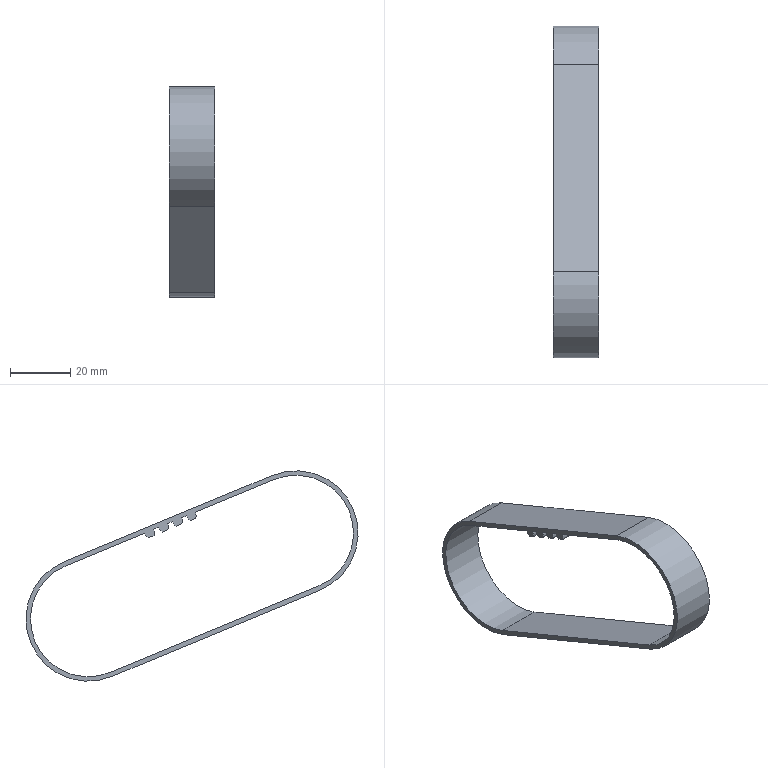Part | NX | features 5003_013_C-HTBN270S5M-150(Default) 2 | 1 solid | 26 faces | box 15 x 109.992 x 69.695 mm | volume 6484 mm3 | plane 14 | cylinder 12 | commonest cylinder face diameters 6.5 x8 38.2 x2 41.2 x2
STEP:
#1=CARTESIAN_POINT('',(-7.975,102.341,-117.355));
#2=VERTEX_POINT('',#1);
#3=CARTESIAN_POINT('',(7.025,102.341,-117.355));
#4=VERTEX_POINT('',#3);
#5=CARTESIAN_POINT('',(-7.975,102.341,-117.355));
#6=DIRECTION('',(1.,0.,0.));
#7=VECTOR('',#6,1000.);
#8=LINE('',#5,#7);
#9=EDGE_CURVE('',#2,#4,#8,.T.);
#10=ORIENTED_EDGE('',*,*,#9,.T.);
#11=CARTESIAN_POINT('',(7.025,100.724,-116.685));
#12=VERTEX_POINT('',#11);
#13=CARTESIAN_POINT('',(7.025,62.517,-100.859));
#14=DIRECTION('',(0.,-0.9239,0.3827));
#15=VECTOR('',#14,1000.);
#16=LINE('',#13,#15);
#17=EDGE_CURVE('',#4,#12,#16,.T.);
#18=ORIENTED_EDGE('',*,*,#17,.T.);
#19=CARTESIAN_POINT('',(-7.975,100.724,-116.685));
#20=VERTEX_POINT('',#19);
#21=CARTESIAN_POINT('',(-7.975,100.724,-116.685));
#22=DIRECTION('',(1.,0.,0.));
#23=VECTOR('',#22,1000.);
#24=LINE('',#21,#23);
#25=EDGE_CURVE('',#20,#12,#24,.T.);
#26=ORIENTED_EDGE('',*,*,#25,.F.);
#27=CARTESIAN_POINT('',(-7.975,62.517,-100.859));
#28=DIRECTION('',(0.,-0.9239,0.3827));
#29=VECTOR('',#28,1000.);
#30=LINE('',#27,#29);
#31=EDGE_CURVE('',#2,#20,#30,.T.);
#32=ORIENTED_EDGE('',*,*,#31,.F.);
#33=EDGE_LOOP('',(#10,#18,#26,#32));
#34=FACE_BOUND('',#33,.T.);
#35=CARTESIAN_POINT('',(7.025,62.517,-100.859));
#36=DIRECTION('',(0.,-0.3827,-0.9239));
#37=DIRECTION('',(-1.,0.,0.));
#38=AXIS2_PLACEMENT_3D('',#35,#36,#37);
#39=PLANE('',#38);
#40=ADVANCED_FACE('',(#34),#39,.T.);
#41=CARTESIAN_POINT('',(-7.975,97.722,-115.441));
#42=VERTEX_POINT('',#41);
#43=CARTESIAN_POINT('',(7.025,97.722,-115.441));
#44=VERTEX_POINT('',#43);
#45=CARTESIAN_POINT('',(-7.975,97.722,-115.441));
#46=DIRECTION('',(1.,0.,0.));
#47=VECTOR('',#46,1000.);
#48=LINE('',#45,#47);
#49=EDGE_CURVE('',#42,#44,#48,.T.);
#50=ORIENTED_EDGE('',*,*,#49,.T.);
#51=CARTESIAN_POINT('',(7.025,96.105,-114.772));
#52=VERTEX_POINT('',#51);
#53=CARTESIAN_POINT('',(7.025,62.517,-100.859));
#54=DIRECTION('',(0.,-0.9239,0.3827));
#55=VECTOR('',#54,1000.);
#56=LINE('',#53,#55);
#57=EDGE_CURVE('',#44,#52,#56,.T.);
#58=ORIENTED_EDGE('',*,*,#57,.T.);
#59=CARTESIAN_POINT('',(-7.975,96.105,-114.772));
#60=VERTEX_POINT('',#59);
#61=CARTESIAN_POINT('',(-7.975,96.105,-114.772));
#62=DIRECTION('',(1.,0.,0.));
#63=VECTOR('',#62,1000.);
#64=LINE('',#61,#63);
#65=EDGE_CURVE('',#60,#52,#64,.T.);
#66=ORIENTED_EDGE('',*,*,#65,.F.);
#67=CARTESIAN_POINT('',(-7.975,62.517,-100.859));
#68=DIRECTION('',(0.,-0.9239,0.3827));
#69=VECTOR('',#68,1000.);
#70=LINE('',#67,#69);
#71=EDGE_CURVE('',#42,#60,#70,.T.);
#72=ORIENTED_EDGE('',*,*,#71,.F.);
#73=EDGE_LOOP('',(#50,#58,#66,#72));
#74=FACE_BOUND('',#73,.T.);
#75=CARTESIAN_POINT('',(7.025,62.517,-100.859));
#76=DIRECTION('',(0.,-0.3827,-0.9239));
#77=DIRECTION('',(-1.,0.,0.));
#78=AXIS2_PLACEMENT_3D('',#75,#76,#77);
#79=PLANE('',#78);
#80=ADVANCED_FACE('',(#74),#79,.T.);
#81=CARTESIAN_POINT('',(-7.975,93.102,-113.528));
#82=VERTEX_POINT('',#81);
#83=CARTESIAN_POINT('',(7.025,93.102,-113.528));
#84=VERTEX_POINT('',#83);
#85=CARTESIAN_POINT('',(-7.975,93.102,-113.528));
#86=DIRECTION('',(1.,0.,0.));
#87=VECTOR('',#86,1000.);
#88=LINE('',#85,#87);
#89=EDGE_CURVE('',#82,#84,#88,.T.);
#90=ORIENTED_EDGE('',*,*,#89,.T.);
#91=CARTESIAN_POINT('',(7.025,91.485,-112.858));
#92=VERTEX_POINT('',#91);
#93=CARTESIAN_POINT('',(7.025,62.517,-100.859));
#94=DIRECTION('',(0.,-0.9239,0.3827));
#95=VECTOR('',#94,1000.);
#96=LINE('',#93,#95);
#97=EDGE_CURVE('',#84,#92,#96,.T.);
#98=ORIENTED_EDGE('',*,*,#97,.T.);
#99=CARTESIAN_POINT('',(-7.975,91.485,-112.858));
#100=VERTEX_POINT('',#99);
#101=CARTESIAN_POINT('',(-7.975,91.485,-112.858));
#102=DIRECTION('',(1.,0.,0.));
#103=VECTOR('',#102,1000.);
#104=LINE('',#101,#103);
#105=EDGE_CURVE('',#100,#92,#104,.T.);
#106=ORIENTED_EDGE('',*,*,#105,.F.);
#107=CARTESIAN_POINT('',(-7.975,62.517,-100.859));
#108=DIRECTION('',(0.,-0.9239,0.3827));
#109=VECTOR('',#108,1000.);
#110=LINE('',#107,#109);
#111=EDGE_CURVE('',#82,#100,#110,.T.);
#112=ORIENTED_EDGE('',*,*,#111,.F.);
#113=EDGE_LOOP('',(#90,#98,#106,#112));
#114=FACE_BOUND('',#113,.T.);
#115=CARTESIAN_POINT('',(7.025,62.517,-100.859));
#116=DIRECTION('',(0.,-0.3827,-0.9239));
#117=DIRECTION('',(-1.,0.,0.));
#118=AXIS2_PLACEMENT_3D('',#115,#116,#117);
#119=PLANE('',#118);
#120=ADVANCED_FACE('',(#114),#119,.T.);
#121=CARTESIAN_POINT('',(-7.975,88.483,-111.615));
#122=VERTEX_POINT('',#121);
#123=CARTESIAN_POINT('',(7.025,88.483,-111.615));
#124=VERTEX_POINT('',#123);
#125=CARTESIAN_POINT('',(-7.975,88.483,-111.615));
#126=DIRECTION('',(1.,0.,0.));
#127=VECTOR('',#126,1000.);
#128=LINE('',#125,#127);
#129=EDGE_CURVE('',#122,#124,#128,.T.);
#130=ORIENTED_EDGE('',*,*,#129,.T.);
#131=CARTESIAN_POINT('',(7.025,62.517,-100.859));
#132=VERTEX_POINT('',#131);
#133=CARTESIAN_POINT('',(7.025,62.517,-100.859));
#134=DIRECTION('',(0.,-0.9239,0.3827));
#135=VECTOR('',#134,1000.);
#136=LINE('',#133,#135);
#137=EDGE_CURVE('',#124,#132,#136,.T.);
#138=ORIENTED_EDGE('',*,*,#137,.T.);
#139=CARTESIAN_POINT('',(-7.975,62.517,-100.859));
#140=VERTEX_POINT('',#139);
#141=CARTESIAN_POINT('',(7.025,62.517,-100.859));
#142=DIRECTION('',(-1.,0.,0.));
#143=VECTOR('',#142,1000.);
#144=LINE('',#141,#143);
#145=EDGE_CURVE('',#132,#140,#144,.T.);
#146=ORIENTED_EDGE('',*,*,#145,.T.);
#147=CARTESIAN_POINT('',(-7.975,62.517,-100.859));
#148=DIRECTION('',(0.,-0.9239,0.3827));
#149=VECTOR('',#148,1000.);
#150=LINE('',#147,#149);
#151=EDGE_CURVE('',#122,#140,#150,.T.);
#152=ORIENTED_EDGE('',*,*,#151,.F.);
#153=EDGE_LOOP('',(#130,#138,#146,#152));
#154=FACE_BOUND('',#153,.T.);
#155=CARTESIAN_POINT('',(7.025,62.517,-100.859));
#156=DIRECTION('',(0.,-0.3827,-0.9239));
#157=DIRECTION('',(-1.,0.,0.));
#158=AXIS2_PLACEMENT_3D('',#155,#156,#157);
#159=PLANE('',#158);
#160=ADVANCED_FACE('',(#154),#159,.T.);
#161=CARTESIAN_POINT('',(7.025,63.091,-99.473));
#162=VERTEX_POINT('',#161);
#163=CARTESIAN_POINT('',(7.025,47.325,-137.537));
#164=VERTEX_POINT('',#163);
#165=CARTESIAN_POINT('',(7.025,55.208,-118.505));
#166=DIRECTION('',(1.,0.,0.));
#167=DIRECTION('',(0.,0.9239,-0.3827));
#168=AXIS2_PLACEMENT_3D('',#165,#166,#167);
#169=CIRCLE('',#168,20.6);
#170=EDGE_CURVE('',#162,#164,#169,.T.);
#171=ORIENTED_EDGE('',*,*,#170,.T.);
#172=CARTESIAN_POINT('',(7.025,116.117,-166.032));
#173=VERTEX_POINT('',#172);
#174=CARTESIAN_POINT('',(7.025,47.325,-137.537));
#175=DIRECTION('',(0.,0.9239,-0.3827));
#176=VECTOR('',#175,1000.);
#177=LINE('',#174,#176);
#178=EDGE_CURVE('',#164,#173,#177,.T.);
#179=ORIENTED_EDGE('',*,*,#178,.T.);
#180=CARTESIAN_POINT('',(7.025,131.883,-127.968));
#181=VERTEX_POINT('',#180);
#182=CARTESIAN_POINT('',(7.025,124.,-147.));
#183=DIRECTION('',(1.,0.,0.));
#184=DIRECTION('',(0.,0.9239,-0.3827));
#185=AXIS2_PLACEMENT_3D('',#182,#183,#184);
#186=CIRCLE('',#185,20.6);
#187=EDGE_CURVE('',#173,#181,#186,.T.);
#188=ORIENTED_EDGE('',*,*,#187,.T.);
#189=CARTESIAN_POINT('',(7.025,63.091,-99.473));
#190=DIRECTION('',(0.,-0.9239,0.3827));
#191=VECTOR('',#190,1000.);
#192=LINE('',#189,#191);
#193=EDGE_CURVE('',#181,#162,#192,.T.);
#194=ORIENTED_EDGE('',*,*,#193,.T.);
#195=EDGE_LOOP('',(#171,#179,#188,#194));
#196=FACE_BOUND('',#195,.T.);
#197=CARTESIAN_POINT('',(7.025,47.899,-136.151));
#198=VERTEX_POINT('',#197);
#199=CARTESIAN_POINT('',(7.025,116.691,-164.646));
#200=VERTEX_POINT('',#199);
#201=CARTESIAN_POINT('',(7.025,47.899,-136.151));
#202=DIRECTION('',(0.,0.9239,-0.3827));
#203=VECTOR('',#202,1000.);
#204=LINE('',#201,#203);
#205=EDGE_CURVE('',#198,#200,#204,.T.);
#206=ORIENTED_EDGE('',*,*,#205,.F.);
#207=CARTESIAN_POINT('',(7.025,55.208,-118.505));
#208=DIRECTION('',(1.,0.,0.));
#209=DIRECTION('',(0.,0.9239,-0.3827));
#210=AXIS2_PLACEMENT_3D('',#207,#208,#209);
#211=CIRCLE('',#210,19.1);
#212=EDGE_CURVE('',#132,#198,#211,.T.);
#213=ORIENTED_EDGE('',*,*,#212,.F.);
#214=ORIENTED_EDGE('',*,*,#137,.F.);
#215=CARTESIAN_POINT('',(7.025,88.325,-113.617));
#216=VERTEX_POINT('',#215);
#217=CARTESIAN_POINT('',(7.025,91.485,-112.858));
#218=DIRECTION('',(1.,0.,0.));
#219=DIRECTION('',(0.,-0.9239,0.3827));
#220=AXIS2_PLACEMENT_3D('',#217,#218,#219);
#221=CIRCLE('',#220,3.25);
#222=EDGE_CURVE('',#124,#216,#221,.T.);
#223=ORIENTED_EDGE('',*,*,#222,.T.);
#224=CARTESIAN_POINT('',(7.025,90.181,-114.385));
#225=VERTEX_POINT('',#224);
#226=CARTESIAN_POINT('',(7.025,90.181,-114.385));
#227=DIRECTION('',(0.,0.9239,-0.3827));
#228=VECTOR('',#227,1000.);
#229=LINE('',#226,#228);
#230=EDGE_CURVE('',#216,#225,#229,.T.);
#231=ORIENTED_EDGE('',*,*,#230,.T.);
#232=CARTESIAN_POINT('',(7.025,88.483,-111.615));
#233=DIRECTION('',(1.,0.,0.));
#234=DIRECTION('',(0.,-0.9239,0.3827));
#235=AXIS2_PLACEMENT_3D('',#232,#233,#234);
#236=CIRCLE('',#235,3.25);
#237=EDGE_CURVE('',#225,#92,#236,.T.);
#238=ORIENTED_EDGE('',*,*,#237,.T.);
#239=ORIENTED_EDGE('',*,*,#97,.F.);
#240=CARTESIAN_POINT('',(7.025,92.945,-115.53));
#241=VERTEX_POINT('',#240);
#242=CARTESIAN_POINT('',(7.025,96.105,-114.772));
#243=DIRECTION('',(1.,0.,0.));
#244=DIRECTION('',(0.,0.9239,-0.3827));
#245=AXIS2_PLACEMENT_3D('',#242,#243,#244);
#246=CIRCLE('',#245,3.25);
#247=EDGE_CURVE('',#84,#241,#246,.T.);
#248=ORIENTED_EDGE('',*,*,#247,.T.);
#249=CARTESIAN_POINT('',(7.025,94.801,-116.299));
#250=VERTEX_POINT('',#249);
#251=CARTESIAN_POINT('',(7.025,92.945,-115.53));
#252=DIRECTION('',(0.,0.9239,-0.3827));
#253=VECTOR('',#252,1000.);
#254=LINE('',#251,#253);
#255=EDGE_CURVE('',#241,#250,#254,.T.);
#256=ORIENTED_EDGE('',*,*,#255,.T.);
#257=CARTESIAN_POINT('',(7.025,93.102,-113.528));
#258=DIRECTION('',(1.,0.,0.));
#259=DIRECTION('',(0.,0.9239,-0.3827));
#260=AXIS2_PLACEMENT_3D('',#257,#258,#259);
#261=CIRCLE('',#260,3.25);
#262=EDGE_CURVE('',#250,#52,#261,.T.);
#263=ORIENTED_EDGE('',*,*,#262,.T.);
#264=ORIENTED_EDGE('',*,*,#57,.F.);
#265=CARTESIAN_POINT('',(7.025,97.564,-117.444));
#266=VERTEX_POINT('',#265);
#267=CARTESIAN_POINT('',(7.025,100.724,-116.685));
#268=DIRECTION('',(1.,0.,0.));
#269=DIRECTION('',(0.,-0.9239,0.3827));
#270=AXIS2_PLACEMENT_3D('',#267,#268,#269);
#271=CIRCLE('',#270,3.25);
#272=EDGE_CURVE('',#44,#266,#271,.T.);
#273=ORIENTED_EDGE('',*,*,#272,.T.);
#274=CARTESIAN_POINT('',(7.025,99.42,-118.212));
#275=VERTEX_POINT('',#274);
#276=CARTESIAN_POINT('',(7.025,99.42,-118.212));
#277=DIRECTION('',(0.,0.9239,-0.3827));
#278=VECTOR('',#277,1000.);
#279=LINE('',#276,#278);
#280=EDGE_CURVE('',#266,#275,#279,.T.);
#281=ORIENTED_EDGE('',*,*,#280,.T.);
#282=CARTESIAN_POINT('',(7.025,97.722,-115.441));
#283=DIRECTION('',(1.,0.,0.));
#284=DIRECTION('',(0.,-0.9239,0.3827));
#285=AXIS2_PLACEMENT_3D('',#282,#283,#284);
#286=CIRCLE('',#285,3.25);
#287=EDGE_CURVE('',#275,#12,#286,.T.);
#288=ORIENTED_EDGE('',*,*,#287,.T.);
#289=ORIENTED_EDGE('',*,*,#17,.F.);
#290=CARTESIAN_POINT('',(7.025,102.183,-119.357));
#291=VERTEX_POINT('',#290);
#292=CARTESIAN_POINT('',(7.025,105.344,-118.599));
#293=DIRECTION('',(1.,0.,0.));
#294=DIRECTION('',(0.,0.9239,-0.3827));
#295=AXIS2_PLACEMENT_3D('',#292,#293,#294);
#296=CIRCLE('',#295,3.25);
#297=EDGE_CURVE('',#4,#291,#296,.T.);
#298=ORIENTED_EDGE('',*,*,#297,.T.);
#299=CARTESIAN_POINT('',(7.025,104.039,-120.126));
#300=VERTEX_POINT('',#299);
#301=CARTESIAN_POINT('',(7.025,102.183,-119.357));
#302=DIRECTION('',(0.,0.9239,-0.3827));
#303=VECTOR('',#302,1000.);
#304=LINE('',#301,#303);
#305=EDGE_CURVE('',#291,#300,#304,.T.);
#306=ORIENTED_EDGE('',*,*,#305,.T.);
#307=CARTESIAN_POINT('',(7.025,105.344,-118.599));
#308=VERTEX_POINT('',#307);
#309=CARTESIAN_POINT('',(7.025,102.341,-117.355));
#310=DIRECTION('',(1.,0.,0.));
#311=DIRECTION('',(0.,0.9239,-0.3827));
#312=AXIS2_PLACEMENT_3D('',#309,#310,#311);
#313=CIRCLE('',#312,3.25);
#314=EDGE_CURVE('',#300,#308,#313,.T.);
#315=ORIENTED_EDGE('',*,*,#314,.T.);
#316=CARTESIAN_POINT('',(7.025,131.309,-129.354));
#317=VERTEX_POINT('',#316);
#318=CARTESIAN_POINT('',(7.025,62.517,-100.859));
#319=DIRECTION('',(0.,-0.9239,0.3827));
#320=VECTOR('',#319,1000.);
#321=LINE('',#318,#320);
#322=EDGE_CURVE('',#317,#308,#321,.T.);
#323=ORIENTED_EDGE('',*,*,#322,.F.);
#324=CARTESIAN_POINT('',(7.025,124.,-147.));
#325=DIRECTION('',(1.,0.,0.));
#326=DIRECTION('',(0.,0.9239,-0.3827));
#327=AXIS2_PLACEMENT_3D('',#324,#325,#326);
#328=CIRCLE('',#327,19.1);
#329=EDGE_CURVE('',#200,#317,#328,.T.);
#330=ORIENTED_EDGE('',*,*,#329,.F.);
#331=EDGE_LOOP('',(#206,#213,#214,#223,#231,#238,#239,#248,#256,#263,#264,#273,#281,#288,#289,#298,#306,#315,#323,#330));
#332=FACE_BOUND('',#331,.T.);
#333=CARTESIAN_POINT('',(7.025,55.208,-118.505));
#334=DIRECTION('',(1.,0.,0.));
#335=DIRECTION('',(0.,0.9239,-0.3827));
#336=AXIS2_PLACEMENT_3D('',#333,#334,#335);
#337=PLANE('',#336);
#338=ADVANCED_FACE('',(#196,#332),#337,.T.);
#339=CARTESIAN_POINT('',(-7.975,63.091,-99.473));
#340=VERTEX_POINT('',#339);
#341=CARTESIAN_POINT('',(-7.975,47.325,-137.537));
#342=VERTEX_POINT('',#341);
#343=CARTESIAN_POINT('',(-7.975,55.208,-118.505));
#344=DIRECTION('',(1.,0.,0.));
#345=DIRECTION('',(0.,0.9239,-0.3827));
#346=AXIS2_PLACEMENT_3D('',#343,#344,#345);
#347=CIRCLE('',#346,20.6);
#348=EDGE_CURVE('',#340,#342,#347,.T.);
#349=ORIENTED_EDGE('',*,*,#348,.F.);
#350=CARTESIAN_POINT('',(-7.975,131.883,-127.968));
#351=VERTEX_POINT('',#350);
#352=CARTESIAN_POINT('',(-7.975,63.091,-99.473));
#353=DIRECTION('',(0.,-0.9239,0.3827));
#354=VECTOR('',#353,1000.);
#355=LINE('',#352,#354);
#356=EDGE_CURVE('',#351,#340,#355,.T.);
#357=ORIENTED_EDGE('',*,*,#356,.F.);
#358=CARTESIAN_POINT('',(-7.975,116.117,-166.032));
#359=VERTEX_POINT('',#358);
#360=CARTESIAN_POINT('',(-7.975,124.,-147.));
#361=DIRECTION('',(1.,0.,0.));
#362=DIRECTION('',(0.,0.9239,-0.3827));
#363=AXIS2_PLACEMENT_3D('',#360,#361,#362);
#364=CIRCLE('',#363,20.6);
#365=EDGE_CURVE('',#359,#351,#364,.T.);
#366=ORIENTED_EDGE('',*,*,#365,.F.);
#367=CARTESIAN_POINT('',(-7.975,47.325,-137.537));
#368=DIRECTION('',(0.,0.9239,-0.3827));
#369=VECTOR('',#368,1000.);
#370=LINE('',#367,#369);
#371=EDGE_CURVE('',#342,#359,#370,.T.);
#372=ORIENTED_EDGE('',*,*,#371,.F.);
#373=EDGE_LOOP('',(#349,#357,#366,#372));
#374=FACE_BOUND('',#373,.T.);
#375=CARTESIAN_POINT('',(-7.975,47.899,-136.151));
#376=VERTEX_POINT('',#375);
#377=CARTESIAN_POINT('',(-7.975,55.208,-118.505));
#378=DIRECTION('',(1.,0.,0.));
#379=DIRECTION('',(0.,0.9239,-0.3827));
#380=AXIS2_PLACEMENT_3D('',#377,#378,#379);
#381=CIRCLE('',#380,19.1);
#382=EDGE_CURVE('',#140,#376,#381,.T.);
#383=ORIENTED_EDGE('',*,*,#382,.T.);
#384=CARTESIAN_POINT('',(-7.975,116.691,-164.646));
#385=VERTEX_POINT('',#384);
#386=CARTESIAN_POINT('',(-7.975,47.899,-136.151));
#387=DIRECTION('',(0.,0.9239,-0.3827));
#388=VECTOR('',#387,1000.);
#389=LINE('',#386,#388);
#390=EDGE_CURVE('',#376,#385,#389,.T.);
#391=ORIENTED_EDGE('',*,*,#390,.T.);
#392=CARTESIAN_POINT('',(-7.975,131.309,-129.354));
#393=VERTEX_POINT('',#392);
#394=CARTESIAN_POINT('',(-7.975,124.,-147.));
#395=DIRECTION('',(1.,0.,0.));
#396=DIRECTION('',(0.,0.9239,-0.3827));
#397=AXIS2_PLACEMENT_3D('',#394,#395,#396);
#398=CIRCLE('',#397,19.1);
#399=EDGE_CURVE('',#385,#393,#398,.T.);
#400=ORIENTED_EDGE('',*,*,#399,.T.);
#401=CARTESIAN_POINT('',(-7.975,105.344,-118.599));
#402=VERTEX_POINT('',#401);
#403=CARTESIAN_POINT('',(-7.975,62.517,-100.859));
#404=DIRECTION('',(0.,-0.9239,0.3827));
#405=VECTOR('',#404,1000.);
#406=LINE('',#403,#405);
#407=EDGE_CURVE('',#393,#402,#406,.T.);
#408=ORIENTED_EDGE('',*,*,#407,.T.);
#409=CARTESIAN_POINT('',(-7.975,104.039,-120.126));
#410=VERTEX_POINT('',#409);
#411=CARTESIAN_POINT('',(-7.975,102.341,-117.355));
#412=DIRECTION('',(1.,0.,0.));
#413=DIRECTION('',(0.,0.9239,-0.3827));
#414=AXIS2_PLACEMENT_3D('',#411,#412,#413);
#415=CIRCLE('',#414,3.25);
#416=EDGE_CURVE('',#410,#402,#415,.T.);
#417=ORIENTED_EDGE('',*,*,#416,.F.);
#418=CARTESIAN_POINT('',(-7.975,102.183,-119.357));
#419=VERTEX_POINT('',#418);
#420=CARTESIAN_POINT('',(-7.975,102.183,-119.357));
#421=DIRECTION('',(0.,0.9239,-0.3827));
#422=VECTOR('',#421,1000.);
#423=LINE('',#420,#422);
#424=EDGE_CURVE('',#419,#410,#423,.T.);
#425=ORIENTED_EDGE('',*,*,#424,.F.);
#426=CARTESIAN_POINT('',(-7.975,105.344,-118.599));
#427=DIRECTION('',(1.,0.,0.));
#428=DIRECTION('',(0.,0.9239,-0.3827));
#429=AXIS2_PLACEMENT_3D('',#426,#427,#428);
#430=CIRCLE('',#429,3.25);
#431=EDGE_CURVE('',#2,#419,#430,.T.);
#432=ORIENTED_EDGE('',*,*,#431,.F.);
#433=ORIENTED_EDGE('',*,*,#31,.T.);
#434=CARTESIAN_POINT('',(-7.975,99.42,-118.212));
#435=VERTEX_POINT('',#434);
#436=CARTESIAN_POINT('',(-7.975,97.722,-115.441));
#437=DIRECTION('',(1.,0.,0.));
#438=DIRECTION('',(0.,-0.9239,0.3827));
#439=AXIS2_PLACEMENT_3D('',#436,#437,#438);
#440=CIRCLE('',#439,3.25);
#441=EDGE_CURVE('',#435,#20,#440,.T.);
#442=ORIENTED_EDGE('',*,*,#441,.F.);
#443=CARTESIAN_POINT('',(-7.975,97.564,-117.444));
#444=VERTEX_POINT('',#443);
#445=CARTESIAN_POINT('',(-7.975,99.42,-118.212));
#446=DIRECTION('',(0.,0.9239,-0.3827));
#447=VECTOR('',#446,1000.);
#448=LINE('',#445,#447);
#449=EDGE_CURVE('',#444,#435,#448,.T.);
#450=ORIENTED_EDGE('',*,*,#449,.F.);
#451=CARTESIAN_POINT('',(-7.975,100.724,-116.685));
#452=DIRECTION('',(1.,0.,0.));
#453=DIRECTION('',(0.,-0.9239,0.3827));
#454=AXIS2_PLACEMENT_3D('',#451,#452,#453);
#455=CIRCLE('',#454,3.25);
#456=EDGE_CURVE('',#42,#444,#455,.T.);
#457=ORIENTED_EDGE('',*,*,#456,.F.);
#458=ORIENTED_EDGE('',*,*,#71,.T.);
#459=CARTESIAN_POINT('',(-7.975,94.801,-116.299));
#460=VERTEX_POINT('',#459);
#461=CARTESIAN_POINT('',(-7.975,93.102,-113.528));
#462=DIRECTION('',(1.,0.,0.));
#463=DIRECTION('',(0.,0.9239,-0.3827));
#464=AXIS2_PLACEMENT_3D('',#461,#462,#463);
#465=CIRCLE('',#464,3.25);
#466=EDGE_CURVE('',#460,#60,#465,.T.);
#467=ORIENTED_EDGE('',*,*,#466,.F.);
#468=CARTESIAN_POINT('',(-7.975,92.945,-115.53));
#469=VERTEX_POINT('',#468);
#470=CARTESIAN_POINT('',(-7.975,92.945,-115.53));
#471=DIRECTION('',(0.,0.9239,-0.3827));
#472=VECTOR('',#471,1000.);
#473=LINE('',#470,#472);
#474=EDGE_CURVE('',#469,#460,#473,.T.);
#475=ORIENTED_EDGE('',*,*,#474,.F.);
#476=CARTESIAN_POINT('',(-7.975,96.105,-114.772));
#477=DIRECTION('',(1.,0.,0.));
#478=DIRECTION('',(0.,0.9239,-0.3827));
#479=AXIS2_PLACEMENT_3D('',#476,#477,#478);
#480=CIRCLE('',#479,3.25);
#481=EDGE_CURVE('',#82,#469,#480,.T.);
#482=ORIENTED_EDGE('',*,*,#481,.F.);
#483=ORIENTED_EDGE('',*,*,#111,.T.);
#484=CARTESIAN_POINT('',(-7.975,90.181,-114.385));
#485=VERTEX_POINT('',#484);
#486=CARTESIAN_POINT('',(-7.975,88.483,-111.615));
#487=DIRECTION('',(1.,0.,0.));
#488=DIRECTION('',(0.,-0.9239,0.3827));
#489=AXIS2_PLACEMENT_3D('',#486,#487,#488);
#490=CIRCLE('',#489,3.25);
#491=EDGE_CURVE('',#485,#100,#490,.T.);
#492=ORIENTED_EDGE('',*,*,#491,.F.);
#493=CARTESIAN_POINT('',(-7.975,88.325,-113.617));
#494=VERTEX_POINT('',#493);
#495=CARTESIAN_POINT('',(-7.975,90.181,-114.385));
#496=DIRECTION('',(0.,0.9239,-0.3827));
#497=VECTOR('',#496,1000.);
#498=LINE('',#495,#497);
#499=EDGE_CURVE('',#494,#485,#498,.T.);
#500=ORIENTED_EDGE('',*,*,#499,.F.);
#501=CARTESIAN_POINT('',(-7.975,91.485,-112.858));
#502=DIRECTION('',(1.,0.,0.));
#503=DIRECTION('',(0.,-0.9239,0.3827));
#504=AXIS2_PLACEMENT_3D('',#501,#502,#503);
#505=CIRCLE('',#504,3.25);
#506=EDGE_CURVE('',#122,#494,#505,.T.);
#507=ORIENTED_EDGE('',*,*,#506,.F.);
#508=ORIENTED_EDGE('',*,*,#151,.T.);
#509=EDGE_LOOP('',(#383,#391,#400,#408,#417,#425,#432,#433,#442,#450,#457,#458,#467,#475,#482,#483,#492,#500,#507,#508));
#510=FACE_BOUND('',#509,.T.);
#511=CARTESIAN_POINT('',(-7.975,55.208,-118.505));
#512=DIRECTION('',(1.,0.,0.));
#513=DIRECTION('',(0.,0.9239,-0.3827));
#514=AXIS2_PLACEMENT_3D('',#511,#512,#513);
#515=PLANE('',#514);
#516=ADVANCED_FACE('',(#374,#510),#515,.F.);
#517=ORIENTED_EDGE('',*,*,#348,.T.);
#518=CARTESIAN_POINT('',(7.025,47.325,-137.537));
#519=DIRECTION('',(-1.,0.,0.));
#520=VECTOR('',#519,1000.);
#521=LINE('',#518,#520);
#522=EDGE_CURVE('',#164,#342,#521,.T.);
#523=ORIENTED_EDGE('',*,*,#522,.F.);
#524=ORIENTED_EDGE('',*,*,#170,.F.);
#525=CARTESIAN_POINT('',(7.025,63.091,-99.473));
#526=DIRECTION('',(-1.,0.,0.));
#527=VECTOR('',#526,1000.);
#528=LINE('',#525,#527);
#529=EDGE_CURVE('',#162,#340,#528,.T.);
#530=ORIENTED_EDGE('',*,*,#529,.T.);
#531=EDGE_LOOP('',(#517,#523,#524,#530));
#532=FACE_BOUND('',#531,.T.);
#533=CARTESIAN_POINT('',(7.025,55.208,-118.505));
#534=DIRECTION('',(-1.,0.,0.));
#535=DIRECTION('',(0.,-0.9239,0.3827));
#536=AXIS2_PLACEMENT_3D('',#533,#534,#535);
#537=CYLINDRICAL_SURFACE('',#536,20.6);
#538=ADVANCED_FACE('',(#532),#537,.T.);
#539=ORIENTED_EDGE('',*,*,#371,.T.);
#540=CARTESIAN_POINT('',(7.025,116.117,-166.032));
#541=DIRECTION('',(-1.,0.,0.));
#542=VECTOR('',#541,1000.);
#543=LINE('',#540,#542);
#544=EDGE_CURVE('',#173,#359,#543,.T.);
#545=ORIENTED_EDGE('',*,*,#544,.F.);
#546=ORIENTED_EDGE('',*,*,#178,.F.);
#547=ORIENTED_EDGE('',*,*,#522,.T.);
#548=EDGE_LOOP('',(#539,#545,#546,#547));
#549=FACE_BOUND('',#548,.T.);
#550=CARTESIAN_POINT('',(7.025,47.325,-137.537));
#551=DIRECTION('',(0.,0.3827,0.9239));
#552=DIRECTION('',(0.,-0.9239,0.3827));
#553=AXIS2_PLACEMENT_3D('',#550,#551,#552);
#554=PLANE('',#553);
#555=ADVANCED_FACE('',(#549),#554,.F.);
#556=ORIENTED_EDGE('',*,*,#365,.T.);
#557=CARTESIAN_POINT('',(7.025,131.883,-127.968));
#558=DIRECTION('',(-1.,0.,0.));
#559=VECTOR('',#558,1000.);
#560=LINE('',#557,#559);
#561=EDGE_CURVE('',#181,#351,#560,.T.);
#562=ORIENTED_EDGE('',*,*,#561,.F.);
#563=ORIENTED_EDGE('',*,*,#187,.F.);
#564=ORIENTED_EDGE('',*,*,#544,.T.);
#565=EDGE_LOOP('',(#556,#562,#563,#564));
#566=FACE_BOUND('',#565,.T.);
#567=CARTESIAN_POINT('',(7.025,124.,-147.));
#568=DIRECTION('',(-1.,0.,0.));
#569=DIRECTION('',(0.,-0.9239,0.3827));
#570=AXIS2_PLACEMENT_3D('',#567,#568,#569);
#571=CYLINDRICAL_SURFACE('',#570,20.6);
#572=ADVANCED_FACE('',(#566),#571,.T.);
#573=ORIENTED_EDGE('',*,*,#356,.T.);
#574=ORIENTED_EDGE('',*,*,#529,.F.);
#575=ORIENTED_EDGE('',*,*,#193,.F.);
#576=ORIENTED_EDGE('',*,*,#561,.T.);
#577=EDGE_LOOP('',(#573,#574,#575,#576));
#578=FACE_BOUND('',#577,.T.);
#579=CARTESIAN_POINT('',(7.025,63.091,-99.473));
#580=DIRECTION('',(0.,-0.3827,-0.9239));
#581=DIRECTION('',(-1.,0.,0.));
#582=AXIS2_PLACEMENT_3D('',#579,#580,#581);
#583=PLANE('',#582);
#584=ADVANCED_FACE('',(#578),#583,.F.);
#585=ORIENTED_EDGE('',*,*,#382,.F.);
#586=ORIENTED_EDGE('',*,*,#145,.F.);
#587=ORIENTED_EDGE('',*,*,#212,.T.);
#588=CARTESIAN_POINT('',(7.025,47.899,-136.151));
#589=DIRECTION('',(-1.,0.,0.));
#590=VECTOR('',#589,1000.);
#591=LINE('',#588,#590);
#592=EDGE_CURVE('',#198,#376,#591,.T.);
#593=ORIENTED_EDGE('',*,*,#592,.T.);
#594=EDGE_LOOP('',(#585,#586,#587,#593));
#595=FACE_BOUND('',#594,.T.);
#596=CARTESIAN_POINT('',(7.025,55.208,-118.505));
#597=DIRECTION('',(-1.,0.,0.));
#598=DIRECTION('',(0.,-0.9239,0.3827));
#599=AXIS2_PLACEMENT_3D('',#596,#597,#598);
#600=CYLINDRICAL_SURFACE('',#599,19.1);
#601=ADVANCED_FACE('',(#595),#600,.F.);
#602=ORIENTED_EDGE('',*,*,#390,.F.);
#603=ORIENTED_EDGE('',*,*,#592,.F.);
#604=ORIENTED_EDGE('',*,*,#205,.T.);
#605=CARTESIAN_POINT('',(7.025,116.691,-164.646));
#606=DIRECTION('',(-1.,0.,0.));
#607=VECTOR('',#606,1000.);
#608=LINE('',#605,#607);
#609=EDGE_CURVE('',#200,#385,#608,.T.);
#610=ORIENTED_EDGE('',*,*,#609,.T.);
#611=EDGE_LOOP('',(#602,#603,#604,#610));
#612=FACE_BOUND('',#611,.T.);
#613=CARTESIAN_POINT('',(7.025,47.899,-136.151));
#614=DIRECTION('',(0.,0.3827,0.9239));
#615=DIRECTION('',(1.,0.,0.));
#616=AXIS2_PLACEMENT_3D('',#613,#614,#615);
#617=PLANE('',#616);
#618=ADVANCED_FACE('',(#612),#617,.T.);
#619=ORIENTED_EDGE('',*,*,#399,.F.);
#620=ORIENTED_EDGE('',*,*,#609,.F.);
#621=ORIENTED_EDGE('',*,*,#329,.T.);
#622=CARTESIAN_POINT('',(7.025,131.309,-129.354));
#623=DIRECTION('',(-1.,0.,0.));
#624=VECTOR('',#623,1000.);
#625=LINE('',#622,#624);
#626=EDGE_CURVE('',#317,#393,#625,.T.);
#627=ORIENTED_EDGE('',*,*,#626,.T.);
#628=EDGE_LOOP('',(#619,#620,#621,#627));
#629=FACE_BOUND('',#628,.T.);
#630=CARTESIAN_POINT('',(7.025,124.,-147.));
#631=DIRECTION('',(-1.,0.,0.));
#632=DIRECTION('',(0.,-0.9239,0.3827));
#633=AXIS2_PLACEMENT_3D('',#630,#631,#632);
#634=CYLINDRICAL_SURFACE('',#633,19.1);
#635=ADVANCED_FACE('',(#629),#634,.F.);
#636=CARTESIAN_POINT('',(-7.975,105.344,-118.599));
#637=DIRECTION('',(1.,0.,0.));
#638=VECTOR('',#637,1000.);
#639=LINE('',#636,#638);
#640=EDGE_CURVE('',#402,#308,#639,.T.);
#641=ORIENTED_EDGE('',*,*,#640,.F.);
#642=ORIENTED_EDGE('',*,*,#407,.F.);
#643=ORIENTED_EDGE('',*,*,#626,.F.);
#644=ORIENTED_EDGE('',*,*,#322,.T.);
#645=EDGE_LOOP('',(#641,#642,#643,#644));
#646=FACE_BOUND('',#645,.T.);
#647=CARTESIAN_POINT('',(7.025,62.517,-100.859));
#648=DIRECTION('',(0.,-0.3827,-0.9239));
#649=DIRECTION('',(-1.,0.,0.));
#650=AXIS2_PLACEMENT_3D('',#647,#648,#649);
#651=PLANE('',#650);
#652=ADVANCED_FACE('',(#646),#651,.T.);
#653=ORIENTED_EDGE('',*,*,#222,.F.);
#654=ORIENTED_EDGE('',*,*,#129,.F.);
#655=ORIENTED_EDGE('',*,*,#506,.T.);
#656=CARTESIAN_POINT('',(-7.975,88.325,-113.617));
#657=DIRECTION('',(1.,0.,0.));
#658=VECTOR('',#657,1000.);
#659=LINE('',#656,#658);
#660=EDGE_CURVE('',#494,#216,#659,.T.);
#661=ORIENTED_EDGE('',*,*,#660,.T.);
#662=EDGE_LOOP('',(#653,#654,#655,#661));
#663=FACE_BOUND('',#662,.T.);
#664=CARTESIAN_POINT('',(-7.975,91.485,-112.858));
#665=DIRECTION('',(1.,0.,0.));
#666=DIRECTION('',(0.,0.9239,-0.3827));
#667=AXIS2_PLACEMENT_3D('',#664,#665,#666);
#668=CYLINDRICAL_SURFACE('',#667,3.25);
#669=ADVANCED_FACE('',(#663),#668,.T.);
#670=ORIENTED_EDGE('',*,*,#237,.F.);
#671=CARTESIAN_POINT('',(-7.975,90.181,-114.385));
#672=DIRECTION('',(1.,0.,0.));
#673=VECTOR('',#672,1000.);
#674=LINE('',#671,#673);
#675=EDGE_CURVE('',#485,#225,#674,.T.);
#676=ORIENTED_EDGE('',*,*,#675,.F.);
#677=ORIENTED_EDGE('',*,*,#491,.T.);
#678=ORIENTED_EDGE('',*,*,#105,.T.);
#679=EDGE_LOOP('',(#670,#676,#677,#678));
#680=FACE_BOUND('',#679,.T.);
#681=CARTESIAN_POINT('',(-7.975,88.483,-111.615));
#682=DIRECTION('',(1.,0.,0.));
#683=DIRECTION('',(0.,0.9239,-0.3827));
#684=AXIS2_PLACEMENT_3D('',#681,#682,#683);
#685=CYLINDRICAL_SURFACE('',#684,3.25);
#686=ADVANCED_FACE('',(#680),#685,.T.);
#687=ORIENTED_EDGE('',*,*,#230,.F.);
#688=ORIENTED_EDGE('',*,*,#660,.F.);
#689=ORIENTED_EDGE('',*,*,#499,.T.);
#690=ORIENTED_EDGE('',*,*,#675,.T.);
#691=EDGE_LOOP('',(#687,#688,#689,#690));
#692=FACE_BOUND('',#691,.T.);
#693=CARTESIAN_POINT('',(-7.975,90.181,-114.385));
#694=DIRECTION('',(0.,-0.3827,-0.9239));
#695=DIRECTION('',(-1.,0.,0.));
#696=AXIS2_PLACEMENT_3D('',#693,#694,#695);
#697=PLANE('',#696);
#698=ADVANCED_FACE('',(#692),#697,.T.);
#699=ORIENTED_EDGE('',*,*,#247,.F.);
#700=ORIENTED_EDGE('',*,*,#89,.F.);
#701=ORIENTED_EDGE('',*,*,#481,.T.);
#702=CARTESIAN_POINT('',(-7.975,92.945,-115.53));
#703=DIRECTION('',(1.,0.,0.));
#704=VECTOR('',#703,1000.);
#705=LINE('',#702,#704);
#706=EDGE_CURVE('',#469,#241,#705,.T.);
#707=ORIENTED_EDGE('',*,*,#706,.T.);
#708=EDGE_LOOP('',(#699,#700,#701,#707));
#709=FACE_BOUND('',#708,.T.);
#710=CARTESIAN_POINT('',(-7.975,96.105,-114.772));
#711=DIRECTION('',(1.,0.,0.));
#712=DIRECTION('',(0.,0.9239,-0.3827));
#713=AXIS2_PLACEMENT_3D('',#710,#711,#712);
#714=CYLINDRICAL_SURFACE('',#713,3.25);
#715=ADVANCED_FACE('',(#709),#714,.T.);
#716=ORIENTED_EDGE('',*,*,#262,.F.);
#717=CARTESIAN_POINT('',(-7.975,94.801,-116.299));
#718=DIRECTION('',(1.,0.,0.));
#719=VECTOR('',#718,1000.);
#720=LINE('',#717,#719);
#721=EDGE_CURVE('',#460,#250,#720,.T.);
#722=ORIENTED_EDGE('',*,*,#721,.F.);
#723=ORIENTED_EDGE('',*,*,#466,.T.);
#724=ORIENTED_EDGE('',*,*,#65,.T.);
#725=EDGE_LOOP('',(#716,#722,#723,#724));
#726=FACE_BOUND('',#725,.T.);
#727=CARTESIAN_POINT('',(-7.975,93.102,-113.528));
#728=DIRECTION('',(1.,0.,0.));
#729=DIRECTION('',(0.,0.9239,-0.3827));
#730=AXIS2_PLACEMENT_3D('',#727,#728,#729);
#731=CYLINDRICAL_SURFACE('',#730,3.25);
#732=ADVANCED_FACE('',(#726),#731,.T.);
#733=ORIENTED_EDGE('',*,*,#255,.F.);
#734=ORIENTED_EDGE('',*,*,#706,.F.);
#735=ORIENTED_EDGE('',*,*,#474,.T.);
#736=ORIENTED_EDGE('',*,*,#721,.T.);
#737=EDGE_LOOP('',(#733,#734,#735,#736));
#738=FACE_BOUND('',#737,.T.);
#739=CARTESIAN_POINT('',(-7.975,92.945,-115.53));
#740=DIRECTION('',(0.,-0.3827,-0.9239));
#741=DIRECTION('',(-1.,0.,0.));
#742=AXIS2_PLACEMENT_3D('',#739,#740,#741);
#743=PLANE('',#742);
#744=ADVANCED_FACE('',(#738),#743,.T.);
#745=ORIENTED_EDGE('',*,*,#272,.F.);
#746=ORIENTED_EDGE('',*,*,#49,.F.);
#747=ORIENTED_EDGE('',*,*,#456,.T.);
#748=CARTESIAN_POINT('',(-7.975,97.564,-117.444));
#749=DIRECTION('',(1.,0.,0.));
#750=VECTOR('',#749,1000.);
#751=LINE('',#748,#750);
#752=EDGE_CURVE('',#444,#266,#751,.T.);
#753=ORIENTED_EDGE('',*,*,#752,.T.);
#754=EDGE_LOOP('',(#745,#746,#747,#753));
#755=FACE_BOUND('',#754,.T.);
#756=CARTESIAN_POINT('',(-7.975,100.724,-116.685));
#757=DIRECTION('',(1.,0.,0.));
#758=DIRECTION('',(0.,0.9239,-0.3827));
#759=AXIS2_PLACEMENT_3D('',#756,#757,#758);
#760=CYLINDRICAL_SURFACE('',#759,3.25);
#761=ADVANCED_FACE('',(#755),#760,.T.);
#762=ORIENTED_EDGE('',*,*,#287,.F.);
#763=CARTESIAN_POINT('',(-7.975,99.42,-118.212));
#764=DIRECTION('',(1.,0.,0.));
#765=VECTOR('',#764,1000.);
#766=LINE('',#763,#765);
#767=EDGE_CURVE('',#435,#275,#766,.T.);
#768=ORIENTED_EDGE('',*,*,#767,.F.);
#769=ORIENTED_EDGE('',*,*,#441,.T.);
#770=ORIENTED_EDGE('',*,*,#25,.T.);
#771=EDGE_LOOP('',(#762,#768,#769,#770));
#772=FACE_BOUND('',#771,.T.);
#773=CARTESIAN_POINT('',(-7.975,97.722,-115.441));
#774=DIRECTION('',(1.,0.,0.));
#775=DIRECTION('',(0.,0.9239,-0.3827));
#776=AXIS2_PLACEMENT_3D('',#773,#774,#775);
#777=CYLINDRICAL_SURFACE('',#776,3.25);
#778=ADVANCED_FACE('',(#772),#777,.T.);
#779=ORIENTED_EDGE('',*,*,#280,.F.);
#780=ORIENTED_EDGE('',*,*,#752,.F.);
#781=ORIENTED_EDGE('',*,*,#449,.T.);
#782=ORIENTED_EDGE('',*,*,#767,.T.);
#783=EDGE_LOOP('',(#779,#780,#781,#782));
#784=FACE_BOUND('',#783,.T.);
#785=CARTESIAN_POINT('',(-7.975,99.42,-118.212));
#786=DIRECTION('',(0.,-0.3827,-0.9239));
#787=DIRECTION('',(-1.,0.,0.));
#788=AXIS2_PLACEMENT_3D('',#785,#786,#787);
#789=PLANE('',#788);
#790=ADVANCED_FACE('',(#784),#789,.T.);
#791=ORIENTED_EDGE('',*,*,#297,.F.);
#792=ORIENTED_EDGE('',*,*,#9,.F.);
#793=ORIENTED_EDGE('',*,*,#431,.T.);
#794=CARTESIAN_POINT('',(-7.975,102.183,-119.357));
#795=DIRECTION('',(1.,0.,0.));
#796=VECTOR('',#795,1000.);
#797=LINE('',#794,#796);
#798=EDGE_CURVE('',#419,#291,#797,.T.);
#799=ORIENTED_EDGE('',*,*,#798,.T.);
#800=EDGE_LOOP('',(#791,#792,#793,#799));
#801=FACE_BOUND('',#800,.T.);
#802=CARTESIAN_POINT('',(-7.975,105.344,-118.599));
#803=DIRECTION('',(1.,0.,0.));
#804=DIRECTION('',(0.,0.9239,-0.3827));
#805=AXIS2_PLACEMENT_3D('',#802,#803,#804);
#806=CYLINDRICAL_SURFACE('',#805,3.25);
#807=ADVANCED_FACE('',(#801),#806,.T.);
#808=ORIENTED_EDGE('',*,*,#314,.F.);
#809=CARTESIAN_POINT('',(-7.975,104.039,-120.126));
#810=DIRECTION('',(1.,0.,0.));
#811=VECTOR('',#810,1000.);
#812=LINE('',#809,#811);
#813=EDGE_CURVE('',#410,#300,#812,.T.);
#814=ORIENTED_EDGE('',*,*,#813,.F.);
#815=ORIENTED_EDGE('',*,*,#416,.T.);
#816=ORIENTED_EDGE('',*,*,#640,.T.);
#817=EDGE_LOOP('',(#808,#814,#815,#816));
#818=FACE_BOUND('',#817,.T.);
#819=CARTESIAN_POINT('',(-7.975,102.341,-117.355));
#820=DIRECTION('',(1.,0.,0.));
#821=DIRECTION('',(0.,0.9239,-0.3827));
#822=AXIS2_PLACEMENT_3D('',#819,#820,#821);
#823=CYLINDRICAL_SURFACE('',#822,3.25);
#824=ADVANCED_FACE('',(#818),#823,.T.);
#825=ORIENTED_EDGE('',*,*,#305,.F.);
#826=ORIENTED_EDGE('',*,*,#798,.F.);
#827=ORIENTED_EDGE('',*,*,#424,.T.);
#828=ORIENTED_EDGE('',*,*,#813,.T.);
#829=EDGE_LOOP('',(#825,#826,#827,#828));
#830=FACE_BOUND('',#829,.T.);
#831=CARTESIAN_POINT('',(-7.975,102.183,-119.357));
#832=DIRECTION('',(0.,-0.3827,-0.9239));
#833=DIRECTION('',(-1.,0.,0.));
#834=AXIS2_PLACEMENT_3D('',#831,#832,#833);
#835=PLANE('',#834);
#836=ADVANCED_FACE('',(#830),#835,.T.);
#837=CLOSED_SHELL('',(#40,#80,#120,#160,#338,#516,#538,#555,#572,#584,#601,#618,#635,#652,#669,#686,#698,#715,#732,#744,#761,#778,#790,#807,#824,#836));
#838=MANIFOLD_SOLID_BREP('',#837);
#839=(LENGTH_UNIT()NAMED_UNIT(*)SI_UNIT(.MILLI.,.METRE.));
#840=UNCERTAINTY_MEASURE_WITH_UNIT(LENGTH_MEASURE(0.00001),#839,'','');
#841=(NAMED_UNIT(*)PLANE_ANGLE_UNIT()SI_UNIT($,.RADIAN.));
#842=(NAMED_UNIT(*)SI_UNIT($,.STERADIAN.)SOLID_ANGLE_UNIT());
#843=(GEOMETRIC_REPRESENTATION_CONTEXT(3)GLOBAL_UNCERTAINTY_ASSIGNED_CONTEXT((#840))GLOBAL_UNIT_ASSIGNED_CONTEXT((#839,#841,#842))REPRESENTATION_CONTEXT('',''));
#844=ADVANCED_BREP_SHAPE_REPRESENTATION('',(#838),#843);